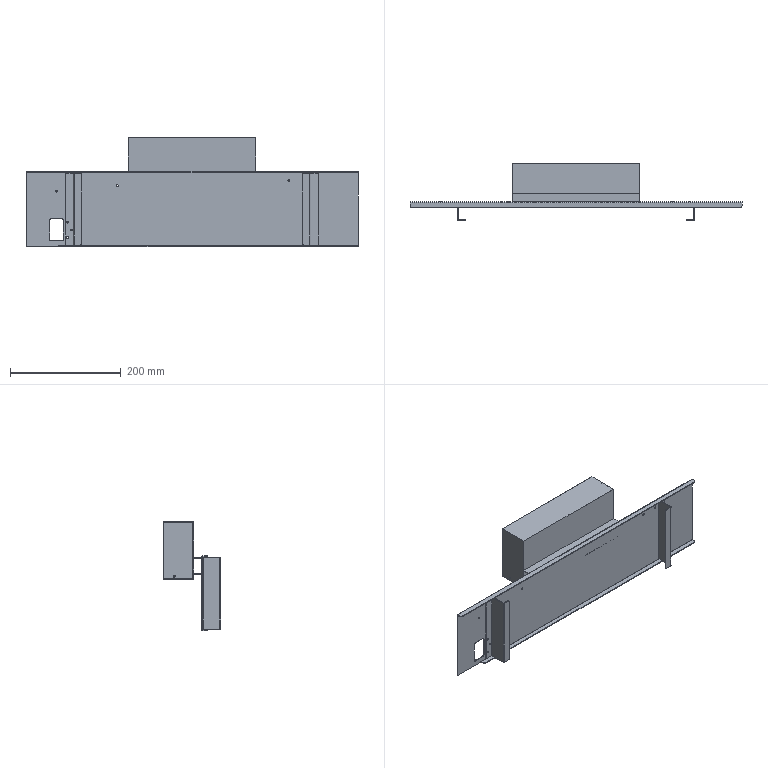Part | SolidWorks | features BaseBody 3 | 3 solids | 126 faces | box 600 x 104 x 197 mm | volume 256427 mm3 | plane 79 | cylinder 47 | commonest cylinder face diameters 3.3 x22 6 x13 0.4 x6 3.4 x6